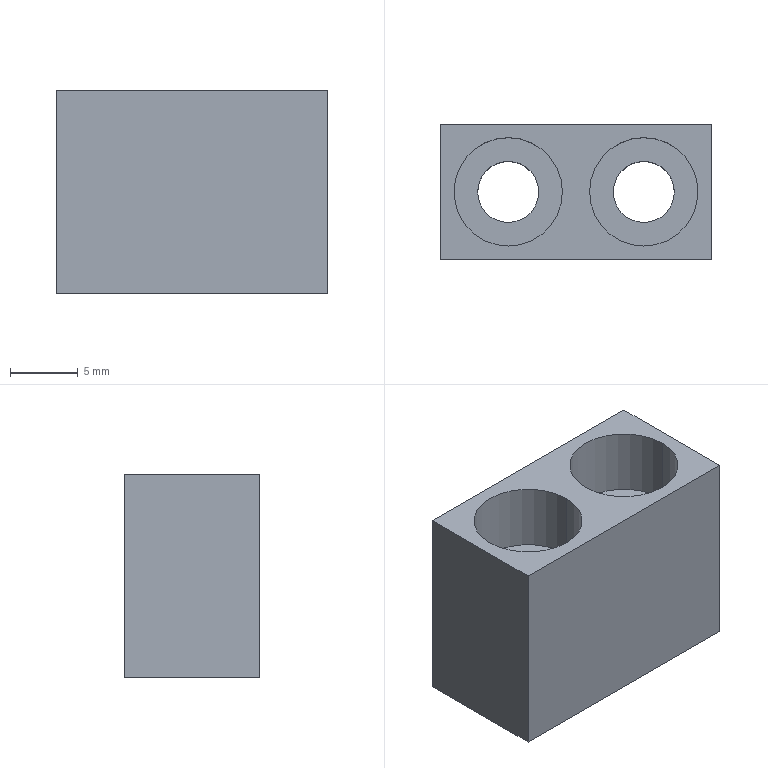Part | STEP file | 227H056259 Stop Block_Default | 1 solid | 16 faces | box 20 x 10 x 15 mm | volume 2179 mm3 | cylinder 8 | plane 8 | commonest cylinder face diameters 4.5 x4 8 x4
STEP:
#1=CARTESIAN_POINT('',(0.,0.,0.));
#2=DIRECTION('',(0.,0.,1.));
#3=DIRECTION('',(1.,0.,0.));
#4=AXIS2_PLACEMENT_3D('',#1,#2,#3);
#5=CARTESIAN_POINT('',(9.,5.,2.5));
#6=VERTEX_POINT('',#5);
#7=CARTESIAN_POINT('',(9.,5.,7.5));
#8=VERTEX_POINT('',#7);
#9=CARTESIAN_POINT('',(9.,5.,7.5));
#10=DIRECTION('',(0.,0.,1.));
#11=VECTOR('',#10,1.);
#12=LINE('',#9,#11);
#13=CARTESIAN_POINT('',(5.,5.,7.5));
#14=DIRECTION('',(0.,0.,1.));
#15=DIRECTION('',(1.,0.,0.));
#16=AXIS2_PLACEMENT_3D('',#13,#14,#15);
#17=CYLINDRICAL_SURFACE('',#16,4.);
#18=CARTESIAN_POINT('',(6.283,0.));
#19=DIRECTION('',(0.,1.));
#20=VECTOR('',#19,1.);
#21=LINE('',#18,#20);
#22=(GEOMETRIC_REPRESENTATION_CONTEXT(2)PARAMETRIC_REPRESENTATION_CONTEXT()REPRESENTATION_CONTEXT('',''));
#23=DEFINITIONAL_REPRESENTATION('',(#21),#22);
#24=PCURVE('',#17,#23);
#25=CARTESIAN_POINT('',(5.,5.,7.5));
#26=DIRECTION('',(0.,0.,1.));
#27=DIRECTION('',(1.,0.,0.));
#28=AXIS2_PLACEMENT_3D('',#25,#26,#27);
#29=CYLINDRICAL_SURFACE('',#28,4.);
#30=CARTESIAN_POINT('',(0.,0.));
#31=DIRECTION('',(0.,1.));
#32=VECTOR('',#31,1.);
#33=LINE('',#30,#32);
#34=(GEOMETRIC_REPRESENTATION_CONTEXT(2)PARAMETRIC_REPRESENTATION_CONTEXT()REPRESENTATION_CONTEXT('',''));
#35=DEFINITIONAL_REPRESENTATION('',(#33),#34);
#36=PCURVE('',#29,#35);
#37=SURFACE_CURVE('',#12,(#24,#36),.PCURVE_S1.);
#38=EDGE_CURVE('',#6,#8,#37,.T.);
#39=ORIENTED_EDGE('',*,*,#38,.T.);
#40=CARTESIAN_POINT('',(1.,5.,7.5));
#41=VERTEX_POINT('',#40);
#42=CARTESIAN_POINT('',(5.,5.,7.5));
#43=DIRECTION('',(0.,0.,1.));
#44=DIRECTION('',(1.,0.,0.));
#45=AXIS2_PLACEMENT_3D('',#42,#43,#44);
#46=CIRCLE('',#45,4.);
#47=CARTESIAN_POINT('',(0.,0.));
#48=DIRECTION('',(1.,0.));
#49=VECTOR('',#48,1.);
#50=LINE('',#47,#49);
#51=(GEOMETRIC_REPRESENTATION_CONTEXT(2)PARAMETRIC_REPRESENTATION_CONTEXT()REPRESENTATION_CONTEXT('',''));
#52=DEFINITIONAL_REPRESENTATION('',(#50),#51);
#53=PCURVE('',#17,#52);
#54=CARTESIAN_POINT('',(10.,10.,7.5));
#55=DIRECTION('',(0.,0.,-1.));
#56=DIRECTION('',(-1.,0.,0.));
#57=AXIS2_PLACEMENT_3D('',#54,#55,#56);
#58=PLANE('',#57);
#59=CARTESIAN_POINT('',(1.,-5.));
#60=CARTESIAN_POINT('',(1.,1.928));
#61=CARTESIAN_POINT('',(7.,-1.536));
#62=CARTESIAN_POINT('',(13.,-5.));
#63=CARTESIAN_POINT('',(7.,-8.464));
#64=CARTESIAN_POINT('',(1.,-11.928));
#65=CARTESIAN_POINT('',(1.,-5.));
#66=(BOUNDED_CURVE()B_SPLINE_CURVE(2,(#59,#60,#61,#62,#63,#64,#65),.UNSPECIFIED.,.T.,.F.)B_SPLINE_CURVE_WITH_KNOTS((1,2,2,2,2,1),(-2.094,0.,2.094,4.189,6.283,8.378),.UNSPECIFIED.)CURVE()GEOMETRIC_REPRESENTATION_ITEM()RATIONAL_B_SPLINE_CURVE((1.,0.5,1.,0.5,1.,0.5,1.))REPRESENTATION_ITEM(''));
#67=(GEOMETRIC_REPRESENTATION_CONTEXT(2)PARAMETRIC_REPRESENTATION_CONTEXT()REPRESENTATION_CONTEXT('',''));
#68=DEFINITIONAL_REPRESENTATION('',(#66),#67);
#69=PCURVE('',#58,#68);
#70=SURFACE_CURVE('',#46,(#53,#69),.PCURVE_S1.);
#71=EDGE_CURVE('',#41,#8,#70,.T.);
#72=ORIENTED_EDGE('',*,*,#71,.F.);
#73=CARTESIAN_POINT('',(1.,5.,2.5));
#74=VERTEX_POINT('',#73);
#75=CARTESIAN_POINT('',(1.,5.,7.5));
#76=DIRECTION('',(0.,0.,1.));
#77=VECTOR('',#76,1.);
#78=LINE('',#75,#77);
#79=CARTESIAN_POINT('',(3.142,0.));
#80=DIRECTION('',(0.,1.));
#81=VECTOR('',#80,1.);
#82=LINE('',#79,#81);
#83=(GEOMETRIC_REPRESENTATION_CONTEXT(2)PARAMETRIC_REPRESENTATION_CONTEXT()REPRESENTATION_CONTEXT('',''));
#84=DEFINITIONAL_REPRESENTATION('',(#82),#83);
#85=PCURVE('',#17,#84);
#86=CARTESIAN_POINT('',(3.142,0.));
#87=DIRECTION('',(0.,1.));
#88=VECTOR('',#87,1.);
#89=LINE('',#86,#88);
#90=(GEOMETRIC_REPRESENTATION_CONTEXT(2)PARAMETRIC_REPRESENTATION_CONTEXT()REPRESENTATION_CONTEXT('',''));
#91=DEFINITIONAL_REPRESENTATION('',(#89),#90);
#92=PCURVE('',#29,#91);
#93=SURFACE_CURVE('',#78,(#85,#92),.PCURVE_S1.);
#94=EDGE_CURVE('',#74,#41,#93,.T.);
#95=ORIENTED_EDGE('',*,*,#94,.F.);
#96=CARTESIAN_POINT('',(5.,5.,2.5));
#97=DIRECTION('',(0.,0.,1.));
#98=DIRECTION('',(1.,0.,0.));
#99=AXIS2_PLACEMENT_3D('',#96,#97,#98);
#100=CIRCLE('',#99,4.);
#101=CARTESIAN_POINT('',(0.,-5.));
#102=DIRECTION('',(1.,0.));
#103=VECTOR('',#102,1.);
#104=LINE('',#101,#103);
#105=(GEOMETRIC_REPRESENTATION_CONTEXT(2)PARAMETRIC_REPRESENTATION_CONTEXT()REPRESENTATION_CONTEXT('',''));
#106=DEFINITIONAL_REPRESENTATION('',(#104),#105);
#107=PCURVE('',#17,#106);
#108=CARTESIAN_POINT('',(7.25,5.,2.5));
#109=DIRECTION('',(0.,0.,-1.));
#110=DIRECTION('',(-1.,0.,0.));
#111=AXIS2_PLACEMENT_3D('',#108,#109,#110);
#112=PLANE('',#111);
#113=CARTESIAN_POINT('',(-1.75,0.));
#114=CARTESIAN_POINT('',(-1.75,6.928));
#115=CARTESIAN_POINT('',(4.25,3.464));
#116=CARTESIAN_POINT('',(10.25,0.));
#117=CARTESIAN_POINT('',(4.25,-3.464));
#118=CARTESIAN_POINT('',(-1.75,-6.928));
#119=CARTESIAN_POINT('',(-1.75,0.));
#120=(BOUNDED_CURVE()B_SPLINE_CURVE(2,(#113,#114,#115,#116,#117,#118,#119),.UNSPECIFIED.,.T.,.F.)B_SPLINE_CURVE_WITH_KNOTS((1,2,2,2,2,1),(-2.094,0.,2.094,4.189,6.283,8.378),.UNSPECIFIED.)CURVE()GEOMETRIC_REPRESENTATION_ITEM()RATIONAL_B_SPLINE_CURVE((1.,0.5,1.,0.5,1.,0.5,1.))REPRESENTATION_ITEM(''));
#121=(GEOMETRIC_REPRESENTATION_CONTEXT(2)PARAMETRIC_REPRESENTATION_CONTEXT()REPRESENTATION_CONTEXT('',''));
#122=DEFINITIONAL_REPRESENTATION('',(#120),#121);
#123=PCURVE('',#112,#122);
#124=SURFACE_CURVE('',#100,(#107,#123),.PCURVE_S1.);
#125=EDGE_CURVE('',#74,#6,#124,.T.);
#126=ORIENTED_EDGE('',*,*,#125,.T.);
#127=EDGE_LOOP('',(#39,#72,#95,#126));
#128=FACE_BOUND('',#127,.F.);
#129=ADVANCED_FACE('',(#128),#17,.F.);
#130=CARTESIAN_POINT('',(7.25,5.,-7.5));
#131=VERTEX_POINT('',#130);
#132=CARTESIAN_POINT('',(7.25,5.,2.5));
#133=VERTEX_POINT('',#132);
#134=CARTESIAN_POINT('',(7.25,5.,7.5));
#135=DIRECTION('',(0.,0.,1.));
#136=VECTOR('',#135,1.);
#137=LINE('',#134,#136);
#138=CARTESIAN_POINT('',(5.,5.,7.5));
#139=DIRECTION('',(0.,0.,1.));
#140=DIRECTION('',(1.,0.,0.));
#141=AXIS2_PLACEMENT_3D('',#138,#139,#140);
#142=CYLINDRICAL_SURFACE('',#141,2.25);
#143=CARTESIAN_POINT('',(6.283,0.));
#144=DIRECTION('',(0.,1.));
#145=VECTOR('',#144,1.);
#146=LINE('',#143,#145);
#147=(GEOMETRIC_REPRESENTATION_CONTEXT(2)PARAMETRIC_REPRESENTATION_CONTEXT()REPRESENTATION_CONTEXT('',''));
#148=DEFINITIONAL_REPRESENTATION('',(#146),#147);
#149=PCURVE('',#142,#148);
#150=CARTESIAN_POINT('',(5.,5.,7.5));
#151=DIRECTION('',(0.,0.,1.));
#152=DIRECTION('',(1.,0.,0.));
#153=AXIS2_PLACEMENT_3D('',#150,#151,#152);
#154=CYLINDRICAL_SURFACE('',#153,2.25);
#155=CARTESIAN_POINT('',(0.,0.));
#156=DIRECTION('',(0.,1.));
#157=VECTOR('',#156,1.);
#158=LINE('',#155,#157);
#159=(GEOMETRIC_REPRESENTATION_CONTEXT(2)PARAMETRIC_REPRESENTATION_CONTEXT()REPRESENTATION_CONTEXT('',''));
#160=DEFINITIONAL_REPRESENTATION('',(#158),#159);
#161=PCURVE('',#154,#160);
#162=SURFACE_CURVE('',#137,(#149,#161),.PCURVE_S1.);
#163=EDGE_CURVE('',#131,#133,#162,.T.);
#164=ORIENTED_EDGE('',*,*,#163,.T.);
#165=CARTESIAN_POINT('',(2.75,5.,2.5));
#166=VERTEX_POINT('',#165);
#167=CARTESIAN_POINT('',(5.,5.,2.5));
#168=DIRECTION('',(0.,0.,1.));
#169=DIRECTION('',(1.,0.,0.));
#170=AXIS2_PLACEMENT_3D('',#167,#168,#169);
#171=CIRCLE('',#170,2.25);
#172=CARTESIAN_POINT('',(0.,-5.));
#173=DIRECTION('',(1.,0.));
#174=VECTOR('',#173,1.);
#175=LINE('',#172,#174);
#176=(GEOMETRIC_REPRESENTATION_CONTEXT(2)PARAMETRIC_REPRESENTATION_CONTEXT()REPRESENTATION_CONTEXT('',''));
#177=DEFINITIONAL_REPRESENTATION('',(#175),#176);
#178=PCURVE('',#142,#177);
#179=CARTESIAN_POINT('',(0.,0.));
#180=CARTESIAN_POINT('',(0.,3.897));
#181=CARTESIAN_POINT('',(3.375,1.949));
#182=CARTESIAN_POINT('',(6.75,0.));
#183=CARTESIAN_POINT('',(3.375,-1.949));
#184=CARTESIAN_POINT('',(0.,-3.897));
#185=CARTESIAN_POINT('',(0.,0.));
#186=(BOUNDED_CURVE()B_SPLINE_CURVE(2,(#179,#180,#181,#182,#183,#184,#185),.UNSPECIFIED.,.T.,.F.)B_SPLINE_CURVE_WITH_KNOTS((1,2,2,2,2,1),(-2.094,0.,2.094,4.189,6.283,8.378),.UNSPECIFIED.)CURVE()GEOMETRIC_REPRESENTATION_ITEM()RATIONAL_B_SPLINE_CURVE((1.,0.5,1.,0.5,1.,0.5,1.))REPRESENTATION_ITEM(''));
#187=(GEOMETRIC_REPRESENTATION_CONTEXT(2)PARAMETRIC_REPRESENTATION_CONTEXT()REPRESENTATION_CONTEXT('',''));
#188=DEFINITIONAL_REPRESENTATION('',(#186),#187);
#189=PCURVE('',#112,#188);
#190=SURFACE_CURVE('',#171,(#178,#189),.PCURVE_S1.);
#191=EDGE_CURVE('',#166,#133,#190,.T.);
#192=ORIENTED_EDGE('',*,*,#191,.F.);
#193=CARTESIAN_POINT('',(2.75,5.,-7.5));
#194=VERTEX_POINT('',#193);
#195=CARTESIAN_POINT('',(2.75,5.,7.5));
#196=DIRECTION('',(0.,0.,1.));
#197=VECTOR('',#196,1.);
#198=LINE('',#195,#197);
#199=CARTESIAN_POINT('',(3.142,0.));
#200=DIRECTION('',(0.,1.));
#201=VECTOR('',#200,1.);
#202=LINE('',#199,#201);
#203=(GEOMETRIC_REPRESENTATION_CONTEXT(2)PARAMETRIC_REPRESENTATION_CONTEXT()REPRESENTATION_CONTEXT('',''));
#204=DEFINITIONAL_REPRESENTATION('',(#202),#203);
#205=PCURVE('',#142,#204);
#206=CARTESIAN_POINT('',(3.142,0.));
#207=DIRECTION('',(0.,1.));
#208=VECTOR('',#207,1.);
#209=LINE('',#206,#208);
#210=(GEOMETRIC_REPRESENTATION_CONTEXT(2)PARAMETRIC_REPRESENTATION_CONTEXT()REPRESENTATION_CONTEXT('',''));
#211=DEFINITIONAL_REPRESENTATION('',(#209),#210);
#212=PCURVE('',#154,#211);
#213=SURFACE_CURVE('',#198,(#205,#212),.PCURVE_S1.);
#214=EDGE_CURVE('',#194,#166,#213,.T.);
#215=ORIENTED_EDGE('',*,*,#214,.F.);
#216=CARTESIAN_POINT('',(5.,5.,-7.5));
#217=DIRECTION('',(0.,0.,1.));
#218=DIRECTION('',(1.,0.,0.));
#219=AXIS2_PLACEMENT_3D('',#216,#217,#218);
#220=CIRCLE('',#219,2.25);
#221=CARTESIAN_POINT('',(0.,-15.));
#222=DIRECTION('',(1.,0.));
#223=VECTOR('',#222,1.);
#224=LINE('',#221,#223);
#225=(GEOMETRIC_REPRESENTATION_CONTEXT(2)PARAMETRIC_REPRESENTATION_CONTEXT()REPRESENTATION_CONTEXT('',''));
#226=DEFINITIONAL_REPRESENTATION('',(#224),#225);
#227=PCURVE('',#142,#226);
#228=CARTESIAN_POINT('',(10.,10.,-7.5));
#229=DIRECTION('',(0.,0.,1.));
#230=DIRECTION('',(1.,0.,0.));
#231=AXIS2_PLACEMENT_3D('',#228,#229,#230);
#232=PLANE('',#231);
#233=CARTESIAN_POINT('',(-5.,-5.));
#234=DIRECTION('',(1.,0.));
#235=AXIS2_PLACEMENT_2D('',#233,#234);
#236=CIRCLE('',#235,2.25);
#237=(GEOMETRIC_REPRESENTATION_CONTEXT(2)PARAMETRIC_REPRESENTATION_CONTEXT()REPRESENTATION_CONTEXT('',''));
#238=DEFINITIONAL_REPRESENTATION('',(#236),#237);
#239=PCURVE('',#232,#238);
#240=SURFACE_CURVE('',#220,(#227,#239),.PCURVE_S1.);
#241=EDGE_CURVE('',#194,#131,#240,.T.);
#242=ORIENTED_EDGE('',*,*,#241,.T.);
#243=EDGE_LOOP('',(#164,#192,#215,#242));
#244=FACE_BOUND('',#243,.F.);
#245=ADVANCED_FACE('',(#244),#142,.F.);
#246=CARTESIAN_POINT('',(-1.,5.,2.5));
#247=VERTEX_POINT('',#246);
#248=CARTESIAN_POINT('',(-1.,5.,7.5));
#249=VERTEX_POINT('',#248);
#250=CARTESIAN_POINT('',(-1.,5.,7.5));
#251=DIRECTION('',(0.,0.,1.));
#252=VECTOR('',#251,1.);
#253=LINE('',#250,#252);
#254=CARTESIAN_POINT('',(-5.,5.,7.5));
#255=DIRECTION('',(0.,0.,1.));
#256=DIRECTION('',(1.,0.,0.));
#257=AXIS2_PLACEMENT_3D('',#254,#255,#256);
#258=CYLINDRICAL_SURFACE('',#257,4.);
#259=CARTESIAN_POINT('',(6.283,0.));
#260=DIRECTION('',(0.,1.));
#261=VECTOR('',#260,1.);
#262=LINE('',#259,#261);
#263=(GEOMETRIC_REPRESENTATION_CONTEXT(2)PARAMETRIC_REPRESENTATION_CONTEXT()REPRESENTATION_CONTEXT('',''));
#264=DEFINITIONAL_REPRESENTATION('',(#262),#263);
#265=PCURVE('',#258,#264);
#266=CARTESIAN_POINT('',(-5.,5.,7.5));
#267=DIRECTION('',(0.,0.,1.));
#268=DIRECTION('',(1.,0.,0.));
#269=AXIS2_PLACEMENT_3D('',#266,#267,#268);
#270=CYLINDRICAL_SURFACE('',#269,4.);
#271=CARTESIAN_POINT('',(0.,0.));
#272=DIRECTION('',(0.,1.));
#273=VECTOR('',#272,1.);
#274=LINE('',#271,#273);
#275=(GEOMETRIC_REPRESENTATION_CONTEXT(2)PARAMETRIC_REPRESENTATION_CONTEXT()REPRESENTATION_CONTEXT('',''));
#276=DEFINITIONAL_REPRESENTATION('',(#274),#275);
#277=PCURVE('',#270,#276);
#278=SURFACE_CURVE('',#253,(#265,#277),.PCURVE_S1.);
#279=EDGE_CURVE('',#247,#249,#278,.T.);
#280=ORIENTED_EDGE('',*,*,#279,.T.);
#281=CARTESIAN_POINT('',(-9.,5.,7.5));
#282=VERTEX_POINT('',#281);
#283=CARTESIAN_POINT('',(-5.,5.,7.5));
#284=DIRECTION('',(0.,0.,1.));
#285=DIRECTION('',(1.,0.,0.));
#286=AXIS2_PLACEMENT_3D('',#283,#284,#285);
#287=CIRCLE('',#286,4.);
#288=CARTESIAN_POINT('',(0.,0.));
#289=DIRECTION('',(1.,0.));
#290=VECTOR('',#289,1.);
#291=LINE('',#288,#290);
#292=(GEOMETRIC_REPRESENTATION_CONTEXT(2)PARAMETRIC_REPRESENTATION_CONTEXT()REPRESENTATION_CONTEXT('',''));
#293=DEFINITIONAL_REPRESENTATION('',(#291),#292);
#294=PCURVE('',#258,#293);
#295=CARTESIAN_POINT('',(11.,-5.));
#296=CARTESIAN_POINT('',(11.,1.928));
#297=CARTESIAN_POINT('',(17.,-1.536));
#298=CARTESIAN_POINT('',(23.,-5.));
#299=CARTESIAN_POINT('',(17.,-8.464));
#300=CARTESIAN_POINT('',(11.,-11.928));
#301=CARTESIAN_POINT('',(11.,-5.));
#302=(BOUNDED_CURVE()B_SPLINE_CURVE(2,(#295,#296,#297,#298,#299,#300,#301),.UNSPECIFIED.,.T.,.F.)B_SPLINE_CURVE_WITH_KNOTS((1,2,2,2,2,1),(-2.094,0.,2.094,4.189,6.283,8.378),.UNSPECIFIED.)CURVE()GEOMETRIC_REPRESENTATION_ITEM()RATIONAL_B_SPLINE_CURVE((1.,0.5,1.,0.5,1.,0.5,1.))REPRESENTATION_ITEM(''));
#303=(GEOMETRIC_REPRESENTATION_CONTEXT(2)PARAMETRIC_REPRESENTATION_CONTEXT()REPRESENTATION_CONTEXT('',''));
#304=DEFINITIONAL_REPRESENTATION('',(#302),#303);
#305=PCURVE('',#58,#304);
#306=SURFACE_CURVE('',#287,(#294,#305),.PCURVE_S1.);
#307=EDGE_CURVE('',#282,#249,#306,.T.);
#308=ORIENTED_EDGE('',*,*,#307,.F.);
#309=CARTESIAN_POINT('',(-9.,5.,2.5));
#310=VERTEX_POINT('',#309);
#311=CARTESIAN_POINT('',(-9.,5.,7.5));
#312=DIRECTION('',(0.,0.,1.));
#313=VECTOR('',#312,1.);
#314=LINE('',#311,#313);
#315=CARTESIAN_POINT('',(3.142,0.));
#316=DIRECTION('',(0.,1.));
#317=VECTOR('',#316,1.);
#318=LINE('',#315,#317);
#319=(GEOMETRIC_REPRESENTATION_CONTEXT(2)PARAMETRIC_REPRESENTATION_CONTEXT()REPRESENTATION_CONTEXT('',''));
#320=DEFINITIONAL_REPRESENTATION('',(#318),#319);
#321=PCURVE('',#258,#320);
#322=CARTESIAN_POINT('',(3.142,0.));
#323=DIRECTION('',(0.,1.));
#324=VECTOR('',#323,1.);
#325=LINE('',#322,#324);
#326=(GEOMETRIC_REPRESENTATION_CONTEXT(2)PARAMETRIC_REPRESENTATION_CONTEXT()REPRESENTATION_CONTEXT('',''));
#327=DEFINITIONAL_REPRESENTATION('',(#325),#326);
#328=PCURVE('',#270,#327);
#329=SURFACE_CURVE('',#314,(#321,#328),.PCURVE_S1.);
#330=EDGE_CURVE('',#310,#282,#329,.T.);
#331=ORIENTED_EDGE('',*,*,#330,.F.);
#332=CARTESIAN_POINT('',(-5.,5.,2.5));
#333=DIRECTION('',(0.,0.,1.));
#334=DIRECTION('',(1.,0.,0.));
#335=AXIS2_PLACEMENT_3D('',#332,#333,#334);
#336=CIRCLE('',#335,4.);
#337=CARTESIAN_POINT('',(0.,-5.));
#338=DIRECTION('',(1.,0.));
#339=VECTOR('',#338,1.);
#340=LINE('',#337,#339);
#341=(GEOMETRIC_REPRESENTATION_CONTEXT(2)PARAMETRIC_REPRESENTATION_CONTEXT()REPRESENTATION_CONTEXT('',''));
#342=DEFINITIONAL_REPRESENTATION('',(#340),#341);
#343=PCURVE('',#258,#342);
#344=CARTESIAN_POINT('',(-2.75,5.,2.5));
#345=DIRECTION('',(0.,0.,-1.));
#346=DIRECTION('',(-1.,0.,0.));
#347=AXIS2_PLACEMENT_3D('',#344,#345,#346);
#348=PLANE('',#347);
#349=CARTESIAN_POINT('',(-1.75,0.));
#350=CARTESIAN_POINT('',(-1.75,6.928));
#351=CARTESIAN_POINT('',(4.25,3.464));
#352=CARTESIAN_POINT('',(10.25,0.));
#353=CARTESIAN_POINT('',(4.25,-3.464));
#354=CARTESIAN_POINT('',(-1.75,-6.928));
#355=CARTESIAN_POINT('',(-1.75,0.));
#356=(BOUNDED_CURVE()B_SPLINE_CURVE(2,(#349,#350,#351,#352,#353,#354,#355),.UNSPECIFIED.,.T.,.F.)B_SPLINE_CURVE_WITH_KNOTS((1,2,2,2,2,1),(-2.094,0.,2.094,4.189,6.283,8.378),.UNSPECIFIED.)CURVE()GEOMETRIC_REPRESENTATION_ITEM()RATIONAL_B_SPLINE_CURVE((1.,0.5,1.,0.5,1.,0.5,1.))REPRESENTATION_ITEM(''));
#357=(GEOMETRIC_REPRESENTATION_CONTEXT(2)PARAMETRIC_REPRESENTATION_CONTEXT()REPRESENTATION_CONTEXT('',''));
#358=DEFINITIONAL_REPRESENTATION('',(#356),#357);
#359=PCURVE('',#348,#358);
#360=SURFACE_CURVE('',#336,(#343,#359),.PCURVE_S1.);
#361=EDGE_CURVE('',#310,#247,#360,.T.);
#362=ORIENTED_EDGE('',*,*,#361,.T.);
#363=EDGE_LOOP('',(#280,#308,#331,#362));
#364=FACE_BOUND('',#363,.F.);
#365=ADVANCED_FACE('',(#364),#258,.F.);
#366=CARTESIAN_POINT('',(-2.75,5.,-7.5));
#367=VERTEX_POINT('',#366);
#368=CARTESIAN_POINT('',(-2.75,5.,2.5));
#369=VERTEX_POINT('',#368);
#370=CARTESIAN_POINT('',(-2.75,5.,7.5));
#371=DIRECTION('',(0.,0.,1.));
#372=VECTOR('',#371,1.);
#373=LINE('',#370,#372);
#374=CARTESIAN_POINT('',(-5.,5.,7.5));
#375=DIRECTION('',(0.,0.,1.));
#376=DIRECTION('',(1.,0.,0.));
#377=AXIS2_PLACEMENT_3D('',#374,#375,#376);
#378=CYLINDRICAL_SURFACE('',#377,2.25);
#379=CARTESIAN_POINT('',(6.283,0.));
#380=DIRECTION('',(0.,1.));
#381=VECTOR('',#380,1.);
#382=LINE('',#379,#381);
#383=(GEOMETRIC_REPRESENTATION_CONTEXT(2)PARAMETRIC_REPRESENTATION_CONTEXT()REPRESENTATION_CONTEXT('',''));
#384=DEFINITIONAL_REPRESENTATION('',(#382),#383);
#385=PCURVE('',#378,#384);
#386=CARTESIAN_POINT('',(-5.,5.,7.5));
#387=DIRECTION('',(0.,0.,1.));
#388=DIRECTION('',(1.,0.,0.));
#389=AXIS2_PLACEMENT_3D('',#386,#387,#388);
#390=CYLINDRICAL_SURFACE('',#389,2.25);
#391=CARTESIAN_POINT('',(0.,0.));
#392=DIRECTION('',(0.,1.));
#393=VECTOR('',#392,1.);
#394=LINE('',#391,#393);
#395=(GEOMETRIC_REPRESENTATION_CONTEXT(2)PARAMETRIC_REPRESENTATION_CONTEXT()REPRESENTATION_CONTEXT('',''));
#396=DEFINITIONAL_REPRESENTATION('',(#394),#395);
#397=PCURVE('',#390,#396);
#398=SURFACE_CURVE('',#373,(#385,#397),.PCURVE_S1.);
#399=EDGE_CURVE('',#367,#369,#398,.T.);
#400=ORIENTED_EDGE('',*,*,#399,.T.);
#401=CARTESIAN_POINT('',(-7.25,5.,2.5));
#402=VERTEX_POINT('',#401);
#403=CARTESIAN_POINT('',(-5.,5.,2.5));
#404=DIRECTION('',(0.,0.,1.));
#405=DIRECTION('',(1.,0.,0.));
#406=AXIS2_PLACEMENT_3D('',#403,#404,#405);
#407=CIRCLE('',#406,2.25);
#408=CARTESIAN_POINT('',(0.,-5.));
#409=DIRECTION('',(1.,0.));
#410=VECTOR('',#409,1.);
#411=LINE('',#408,#410);
#412=(GEOMETRIC_REPRESENTATION_CONTEXT(2)PARAMETRIC_REPRESENTATION_CONTEXT()REPRESENTATION_CONTEXT('',''));
#413=DEFINITIONAL_REPRESENTATION('',(#411),#412);
#414=PCURVE('',#378,#413);
#415=CARTESIAN_POINT('',(0.,0.));
#416=CARTESIAN_POINT('',(0.,3.897));
#417=CARTESIAN_POINT('',(3.375,1.949));
#418=CARTESIAN_POINT('',(6.75,0.));
#419=CARTESIAN_POINT('',(3.375,-1.949));
#420=CARTESIAN_POINT('',(0.,-3.897));
#421=CARTESIAN_POINT('',(0.,0.));
#422=(BOUNDED_CURVE()B_SPLINE_CURVE(2,(#415,#416,#417,#418,#419,#420,#421),.UNSPECIFIED.,.T.,.F.)B_SPLINE_CURVE_WITH_KNOTS((1,2,2,2,2,1),(-2.094,0.,2.094,4.189,6.283,8.378),.UNSPECIFIED.)CURVE()GEOMETRIC_REPRESENTATION_ITEM()RATIONAL_B_SPLINE_CURVE((1.,0.5,1.,0.5,1.,0.5,1.))REPRESENTATION_ITEM(''));
#423=(GEOMETRIC_REPRESENTATION_CONTEXT(2)PARAMETRIC_REPRESENTATION_CONTEXT()REPRESENTATION_CONTEXT('',''));
#424=DEFINITIONAL_REPRESENTATION('',(#422),#423);
#425=PCURVE('',#348,#424);
#426=SURFACE_CURVE('',#407,(#414,#425),.PCURVE_S1.);
#427=EDGE_CURVE('',#402,#369,#426,.T.);
#428=ORIENTED_EDGE('',*,*,#427,.F.);
#429=CARTESIAN_POINT('',(-7.25,5.,-7.5));
#430=VERTEX_POINT('',#429);
#431=CARTESIAN_POINT('',(-7.25,5.,7.5));
#432=DIRECTION('',(0.,0.,1.));
#433=VECTOR('',#432,1.);
#434=LINE('',#431,#433);
#435=CARTESIAN_POINT('',(3.142,0.));
#436=DIRECTION('',(0.,1.));
#437=VECTOR('',#436,1.);
#438=LINE('',#435,#437);
#439=(GEOMETRIC_REPRESENTATION_CONTEXT(2)PARAMETRIC_REPRESENTATION_CONTEXT()REPRESENTATION_CONTEXT('',''));
#440=DEFINITIONAL_REPRESENTATION('',(#438),#439);
#441=PCURVE('',#378,#440);
#442=CARTESIAN_POINT('',(3.142,0.));
#443=DIRECTION('',(0.,1.));
#444=VECTOR('',#443,1.);
#445=LINE('',#442,#444);
#446=(GEOMETRIC_REPRESENTATION_CONTEXT(2)PARAMETRIC_REPRESENTATION_CONTEXT()REPRESENTATION_CONTEXT('',''));
#447=DEFINITIONAL_REPRESENTATION('',(#445),#446);
#448=PCURVE('',#390,#447);
#449=SURFACE_CURVE('',#434,(#441,#448),.PCURVE_S1.);
#450=EDGE_CURVE('',#430,#402,#449,.T.);
#451=ORIENTED_EDGE('',*,*,#450,.F.);
#452=CARTESIAN_POINT('',(-5.,5.,-7.5));
#453=DIRECTION('',(0.,0.,1.));
#454=DIRECTION('',(1.,0.,0.));
#455=AXIS2_PLACEMENT_3D('',#452,#453,#454);
#456=CIRCLE('',#455,2.25);
#457=CARTESIAN_POINT('',(0.,-15.));
#458=DIRECTION('',(1.,0.));
#459=VECTOR('',#458,1.);
#460=LINE('',#457,#459);
#461=(GEOMETRIC_REPRESENTATION_CONTEXT(2)PARAMETRIC_REPRESENTATION_CONTEXT()REPRESENTATION_CONTEXT('',''));
#462=DEFINITIONAL_REPRESENTATION('',(#460),#461);
#463=PCURVE('',#378,#462);
#464=CARTESIAN_POINT('',(-15.,-5.));
#465=DIRECTION('',(1.,0.));
#466=AXIS2_PLACEMENT_2D('',#464,#465);
#467=CIRCLE('',#466,2.25);
#468=(GEOMETRIC_REPRESENTATION_CONTEXT(2)PARAMETRIC_REPRESENTATION_CONTEXT()REPRESENTATION_CONTEXT('',''));
#469=DEFINITIONAL_REPRESENTATION('',(#467),#468);
#470=PCURVE('',#232,#469);
#471=SURFACE_CURVE('',#456,(#463,#470),.PCURVE_S1.);
#472=EDGE_CURVE('',#430,#367,#471,.T.);
#473=ORIENTED_EDGE('',*,*,#472,.T.);
#474=EDGE_LOOP('',(#400,#428,#451,#473));
#475=FACE_BOUND('',#474,.F.);
#476=ADVANCED_FACE('',(#475),#378,.F.);
#477=CARTESIAN_POINT('',(-10.,0.,-7.5));
#478=VERTEX_POINT('',#477);
#479=CARTESIAN_POINT('',(-10.,0.,7.5));
#480=VERTEX_POINT('',#479);
#481=CARTESIAN_POINT('',(-10.,0.,7.5));
#482=DIRECTION('',(0.,0.,1.));
#483=VECTOR('',#482,1.);
#484=LINE('',#481,#483);
#485=CARTESIAN_POINT('',(-10.,10.,7.5));
#486=DIRECTION('',(1.,0.,0.));
#487=DIRECTION('',(0.,0.,-1.));
#488=AXIS2_PLACEMENT_3D('',#485,#486,#487);
#489=PLANE('',#488);
#490=CARTESIAN_POINT('',(0.,-10.));
#491=DIRECTION('',(-1.,0.));
#492=VECTOR('',#491,1.);
#493=LINE('',#490,#492);
#494=(GEOMETRIC_REPRESENTATION_CONTEXT(2)PARAMETRIC_REPRESENTATION_CONTEXT()REPRESENTATION_CONTEXT('',''));
#495=DEFINITIONAL_REPRESENTATION('',(#493),#494);
#496=PCURVE('',#489,#495);
#497=CARTESIAN_POINT('',(0.,0.,0.));
#498=DIRECTION('',(0.,1.,0.));
#499=DIRECTION('',(0.,0.,1.));
#500=AXIS2_PLACEMENT_3D('',#497,#498,#499);
#501=PLANE('',#500);
#502=CARTESIAN_POINT('',(7.5,-10.));
#503=DIRECTION('',(1.,0.));
#504=VECTOR('',#503,1.);
#505=LINE('',#502,#504);
#506=(GEOMETRIC_REPRESENTATION_CONTEXT(2)PARAMETRIC_REPRESENTATION_CONTEXT()REPRESENTATION_CONTEXT('',''));
#507=DEFINITIONAL_REPRESENTATION('',(#505),#506);
#508=PCURVE('',#501,#507);
#509=SURFACE_CURVE('',#484,(#496,#508),.PCURVE_S1.);
#510=EDGE_CURVE('',#478,#480,#509,.T.);
#511=ORIENTED_EDGE('',*,*,#510,.T.);
#512=CARTESIAN_POINT('',(-10.,10.,7.5));
#513=VERTEX_POINT('',#512);
#514=CARTESIAN_POINT('',(-10.,10.,7.5));
#515=DIRECTION('',(0.,-1.,0.));
#516=VECTOR('',#515,1.);
#517=LINE('',#514,#516);
#518=CARTESIAN_POINT('',(0.,0.));
#519=DIRECTION('',(0.,-1.));
#520=VECTOR('',#519,1.);
#521=LINE('',#518,#520);
#522=(GEOMETRIC_REPRESENTATION_CONTEXT(2)PARAMETRIC_REPRESENTATION_CONTEXT()REPRESENTATION_CONTEXT('',''));
#523=DEFINITIONAL_REPRESENTATION('',(#521),#522);
#524=PCURVE('',#489,#523);
#525=CARTESIAN_POINT('',(20.,0.));
#526=DIRECTION('',(0.,-1.));
#527=VECTOR('',#526,1.);
#528=LINE('',#525,#527);
#529=(GEOMETRIC_REPRESENTATION_CONTEXT(2)PARAMETRIC_REPRESENTATION_CONTEXT()REPRESENTATION_CONTEXT('',''));
#530=DEFINITIONAL_REPRESENTATION('',(#528),#529);
#531=PCURVE('',#58,#530);
#532=SURFACE_CURVE('',#517,(#524,#531),.PCURVE_S1.);
#533=EDGE_CURVE('',#513,#480,#532,.T.);
#534=ORIENTED_EDGE('',*,*,#533,.F.);
#535=CARTESIAN_POINT('',(-10.,10.,-7.5));
#536=VERTEX_POINT('',#535);
#537=CARTESIAN_POINT('',(-10.,10.,7.5));
#538=DIRECTION('',(0.,0.,1.));
#539=VECTOR('',#538,1.);
#540=LINE('',#537,#539);
#541=CARTESIAN_POINT('',(0.,0.));
#542=DIRECTION('',(-1.,0.));
#543=VECTOR('',#542,1.);
#544=LINE('',#541,#543);
#545=(GEOMETRIC_REPRESENTATION_CONTEXT(2)PARAMETRIC_REPRESENTATION_CONTEXT()REPRESENTATION_CONTEXT('',''));
#546=DEFINITIONAL_REPRESENTATION('',(#544),#545);
#547=PCURVE('',#489,#546);
#548=CARTESIAN_POINT('',(0.,10.,0.));
#549=DIRECTION('',(0.,1.,0.));
#550=DIRECTION('',(0.,0.,1.));
#551=AXIS2_PLACEMENT_3D('',#548,#549,#550);
#552=PLANE('',#551);
#553=CARTESIAN_POINT('',(7.5,-10.));
#554=DIRECTION('',(1.,0.));
#555=VECTOR('',#554,1.);
#556=LINE('',#553,#555);
#557=(GEOMETRIC_REPRESENTATION_CONTEXT(2)PARAMETRIC_REPRESENTATION_CONTEXT()REPRESENTATION_CONTEXT('',''));
#558=DEFINITIONAL_REPRESENTATION('',(#556),#557);
#559=PCURVE('',#552,#558);
#560=SURFACE_CURVE('',#540,(#547,#559),.PCURVE_S1.);
#561=EDGE_CURVE('',#536,#513,#560,.T.);
#562=ORIENTED_EDGE('',*,*,#561,.F.);
#563=CARTESIAN_POINT('',(-10.,10.,-7.5));
#564=DIRECTION('',(0.,-1.,0.));
#565=VECTOR('',#564,1.);
#566=LINE('',#563,#565);
#567=CARTESIAN_POINT('',(15.,0.));
#568=DIRECTION('',(0.,-1.));
#569=VECTOR('',#568,1.);
#570=LINE('',#567,#569);
#571=(GEOMETRIC_REPRESENTATION_CONTEXT(2)PARAMETRIC_REPRESENTATION_CONTEXT()REPRESENTATION_CONTEXT('',''));
#572=DEFINITIONAL_REPRESENTATION('',(#570),#571);
#573=PCURVE('',#489,#572);
#574=CARTESIAN_POINT('',(-20.,0.));
#575=DIRECTION('',(0.,-1.));
#576=VECTOR('',#575,1.);
#577=LINE('',#574,#576);
#578=(GEOMETRIC_REPRESENTATION_CONTEXT(2)PARAMETRIC_REPRESENTATION_CONTEXT()REPRESENTATION_CONTEXT('',''));
#579=DEFINITIONAL_REPRESENTATION('',(#577),#578);
#580=PCURVE('',#232,#579);
#581=SURFACE_CURVE('',#566,(#573,#580),.PCURVE_S1.);
#582=EDGE_CURVE('',#536,#478,#581,.T.);
#583=ORIENTED_EDGE('',*,*,#582,.T.);
#584=EDGE_LOOP('',(#511,#534,#562,#583));
#585=FACE_BOUND('',#584,.T.);
#586=ADVANCED_FACE('',(#585),#489,.F.);
#587=CARTESIAN_POINT('',(5.,5.,7.5));
#588=DIRECTION('',(0.,0.,1.));
#589=DIRECTION('',(1.,0.,0.));
#590=AXIS2_PLACEMENT_3D('',#587,#588,#589);
#591=CIRCLE('',#590,4.);
#592=CARTESIAN_POINT('',(1.,-5.));
#593=CARTESIAN_POINT('',(1.,1.928));
#594=CARTESIAN_POINT('',(7.,-1.536));
#595=CARTESIAN_POINT('',(13.,-5.));
#596=CARTESIAN_POINT('',(7.,-8.464));
#597=CARTESIAN_POINT('',(1.,-11.928));
#598=CARTESIAN_POINT('',(1.,-5.));
#599=(BOUNDED_CURVE()B_SPLINE_CURVE(2,(#592,#593,#594,#595,#596,#597,#598),.UNSPECIFIED.,.T.,.F.)B_SPLINE_CURVE_WITH_KNOTS((1,2,2,2,2,1),(-2.094,0.,2.094,4.189,6.283,8.378),.UNSPECIFIED.)CURVE()GEOMETRIC_REPRESENTATION_ITEM()RATIONAL_B_SPLINE_CURVE((1.,0.5,1.,0.5,1.,0.5,1.))REPRESENTATION_ITEM(''));
#600=(GEOMETRIC_REPRESENTATION_CONTEXT(2)PARAMETRIC_REPRESENTATION_CONTEXT()REPRESENTATION_CONTEXT('',''));
#601=DEFINITIONAL_REPRESENTATION('',(#599),#600);
#602=PCURVE('',#58,#601);
#603=CARTESIAN_POINT('',(0.,0.));
#604=DIRECTION('',(1.,0.));
#605=VECTOR('',#604,1.);
#606=LINE('',#603,#605);
#607=(GEOMETRIC_REPRESENTATION_CONTEXT(2)PARAMETRIC_REPRESENTATION_CONTEXT()REPRESENTATION_CONTEXT('',''));
#608=DEFINITIONAL_REPRESENTATION('',(#606),#607);
#609=PCURVE('',#29,#608);
#610=SURFACE_CURVE('',#591,(#602,#609),.PCURVE_S1.);
#611=EDGE_CURVE('',#8,#41,#610,.T.);
#612=ORIENTED_EDGE('',*,*,#611,.F.);
#613=ORIENTED_EDGE('',*,*,#71,.F.);
#614=EDGE_LOOP('',(#612,#613));
#615=FACE_BOUND('',#614,.T.);
#616=CARTESIAN_POINT('',(-5.,5.,7.5));
#617=DIRECTION('',(0.,0.,1.));
#618=DIRECTION('',(1.,0.,0.));
#619=AXIS2_PLACEMENT_3D('',#616,#617,#618);
#620=CIRCLE('',#619,4.);
#621=CARTESIAN_POINT('',(11.,-5.));
#622=CARTESIAN_POINT('',(11.,1.928));
#623=CARTESIAN_POINT('',(17.,-1.536));
#624=CARTESIAN_POINT('',(23.,-5.));
#625=CARTESIAN_POINT('',(17.,-8.464));
#626=CARTESIAN_POINT('',(11.,-11.928));
#627=CARTESIAN_POINT('',(11.,-5.));
#628=(BOUNDED_CURVE()B_SPLINE_CURVE(2,(#621,#622,#623,#624,#625,#626,#627),.UNSPECIFIED.,.T.,.F.)B_SPLINE_CURVE_WITH_KNOTS((1,2,2,2,2,1),(-2.094,0.,2.094,4.189,6.283,8.378),.UNSPECIFIED.)CURVE()GEOMETRIC_REPRESENTATION_ITEM()RATIONAL_B_SPLINE_CURVE((1.,0.5,1.,0.5,1.,0.5,1.))REPRESENTATION_ITEM(''));
#629=(GEOMETRIC_REPRESENTATION_CONTEXT(2)PARAMETRIC_REPRESENTATION_CONTEXT()REPRESENTATION_CONTEXT('',''));
#630=DEFINITIONAL_REPRESENTATION('',(#628),#629);
#631=PCURVE('',#58,#630);
#632=CARTESIAN_POINT('',(0.,0.));
#633=DIRECTION('',(1.,0.));
#634=VECTOR('',#633,1.);
#635=LINE('',#632,#634);
#636=(GEOMETRIC_REPRESENTATION_CONTEXT(2)PARAMETRIC_REPRESENTATION_CONTEXT()REPRESENTATION_CONTEXT('',''));
#637=DEFINITIONAL_REPRESENTATION('',(#635),#636);
#638=PCURVE('',#270,#637);
#639=SURFACE_CURVE('',#620,(#631,#638),.PCURVE_S1.);
#640=EDGE_CURVE('',#249,#282,#639,.T.);
#641=ORIENTED_EDGE('',*,*,#640,.F.);
#642=ORIENTED_EDGE('',*,*,#307,.F.);
#643=EDGE_LOOP('',(#641,#642));
#644=FACE_BOUND('',#643,.T.);
#645=CARTESIAN_POINT('',(10.,0.,7.5));
#646=VERTEX_POINT('',#645);
#647=CARTESIAN_POINT('',(10.,0.,7.5));
#648=DIRECTION('',(1.,0.,0.));
#649=VECTOR('',#648,1.);
#650=LINE('',#647,#649);
#651=CARTESIAN_POINT('',(0.,-10.));
#652=DIRECTION('',(-1.,0.));
#653=VECTOR('',#652,1.);
#654=LINE('',#651,#653);
#655=(GEOMETRIC_REPRESENTATION_CONTEXT(2)PARAMETRIC_REPRESENTATION_CONTEXT()REPRESENTATION_CONTEXT('',''));
#656=DEFINITIONAL_REPRESENTATION('',(#654),#655);
#657=PCURVE('',#58,#656);
#658=CARTESIAN_POINT('',(7.5,10.));
#659=DIRECTION('',(0.,1.));
#660=VECTOR('',#659,1.);
#661=LINE('',#658,#660);
#662=(GEOMETRIC_REPRESENTATION_CONTEXT(2)PARAMETRIC_REPRESENTATION_CONTEXT()REPRESENTATION_CONTEXT('',''));
#663=DEFINITIONAL_REPRESENTATION('',(#661),#662);
#664=PCURVE('',#501,#663);
#665=SURFACE_CURVE('',#650,(#657,#664),.PCURVE_S1.);
#666=EDGE_CURVE('',#480,#646,#665,.T.);
#667=ORIENTED_EDGE('',*,*,#666,.T.);
#668=CARTESIAN_POINT('',(10.,10.,7.5));
#669=VERTEX_POINT('',#668);
#670=CARTESIAN_POINT('',(10.,10.,7.5));
#671=DIRECTION('',(0.,-1.,0.));
#672=VECTOR('',#671,1.);
#673=LINE('',#670,#672);
#674=CARTESIAN_POINT('',(0.,0.));
#675=DIRECTION('',(0.,-1.));
#676=VECTOR('',#675,1.);
#677=LINE('',#674,#676);
#678=(GEOMETRIC_REPRESENTATION_CONTEXT(2)PARAMETRIC_REPRESENTATION_CONTEXT()REPRESENTATION_CONTEXT('',''));
#679=DEFINITIONAL_REPRESENTATION('',(#677),#678);
#680=PCURVE('',#58,#679);
#681=CARTESIAN_POINT('',(10.,10.,7.5));
#682=DIRECTION('',(-1.,0.,0.));
#683=DIRECTION('',(0.,0.,1.));
#684=AXIS2_PLACEMENT_3D('',#681,#682,#683);
#685=PLANE('',#684);
#686=CARTESIAN_POINT('',(0.,0.));
#687=DIRECTION('',(0.,-1.));
#688=VECTOR('',#687,1.);
#689=LINE('',#686,#688);
#690=(GEOMETRIC_REPRESENTATION_CONTEXT(2)PARAMETRIC_REPRESENTATION_CONTEXT()REPRESENTATION_CONTEXT('',''));
#691=DEFINITIONAL_REPRESENTATION('',(#689),#690);
#692=PCURVE('',#685,#691);
#693=SURFACE_CURVE('',#673,(#680,#692),.PCURVE_S1.);
#694=EDGE_CURVE('',#669,#646,#693,.T.);
#695=ORIENTED_EDGE('',*,*,#694,.F.);
#696=CARTESIAN_POINT('',(10.,10.,7.5));
#697=DIRECTION('',(1.,0.,0.));
#698=VECTOR('',#697,1.);
#699=LINE('',#696,#698);
#700=CARTESIAN_POINT('',(0.,0.));
#701=DIRECTION('',(-1.,0.));
#702=VECTOR('',#701,1.);
#703=LINE('',#700,#702);
#704=(GEOMETRIC_REPRESENTATION_CONTEXT(2)PARAMETRIC_REPRESENTATION_CONTEXT()REPRESENTATION_CONTEXT('',''));
#705=DEFINITIONAL_REPRESENTATION('',(#703),#704);
#706=PCURVE('',#58,#705);
#707=CARTESIAN_POINT('',(7.5,10.));
#708=DIRECTION('',(0.,1.));
#709=VECTOR('',#708,1.);
#710=LINE('',#707,#709);
#711=(GEOMETRIC_REPRESENTATION_CONTEXT(2)PARAMETRIC_REPRESENTATION_CONTEXT()REPRESENTATION_CONTEXT('',''));
#712=DEFINITIONAL_REPRESENTATION('',(#710),#711);
#713=PCURVE('',#552,#712);
#714=SURFACE_CURVE('',#699,(#706,#713),.PCURVE_S1.);
#715=EDGE_CURVE('',#513,#669,#714,.T.);
#716=ORIENTED_EDGE('',*,*,#715,.F.);
#717=ORIENTED_EDGE('',*,*,#533,.T.);
#718=EDGE_LOOP('',(#667,#695,#716,#717));
#719=FACE_BOUND('',#718,.T.);
#720=ADVANCED_FACE('',(#615,#644,#719),#58,.F.);
#721=CARTESIAN_POINT('',(10.,0.,-7.5));
#722=VERTEX_POINT('',#721);
#723=CARTESIAN_POINT('',(10.,0.,7.5));
#724=DIRECTION('',(0.,0.,-1.));
#725=VECTOR('',#724,1.);
#726=LINE('',#723,#725);
#727=CARTESIAN_POINT('',(0.,-10.));
#728=DIRECTION('',(-1.,0.));
#729=VECTOR('',#728,1.);
#730=LINE('',#727,#729);
#731=(GEOMETRIC_REPRESENTATION_CONTEXT(2)PARAMETRIC_REPRESENTATION_CONTEXT()REPRESENTATION_CONTEXT('',''));
#732=DEFINITIONAL_REPRESENTATION('',(#730),#731);
#733=PCURVE('',#685,#732);
#734=CARTESIAN_POINT('',(7.5,10.));
#735=DIRECTION('',(-1.,0.));
#736=VECTOR('',#735,1.);
#737=LINE('',#734,#736);
#738=(GEOMETRIC_REPRESENTATION_CONTEXT(2)PARAMETRIC_REPRESENTATION_CONTEXT()REPRESENTATION_CONTEXT('',''));
#739=DEFINITIONAL_REPRESENTATION('',(#737),#738);
#740=PCURVE('',#501,#739);
#741=SURFACE_CURVE('',#726,(#733,#740),.PCURVE_S1.);
#742=EDGE_CURVE('',#646,#722,#741,.T.);
#743=ORIENTED_EDGE('',*,*,#742,.T.);
#744=CARTESIAN_POINT('',(10.,10.,-7.5));
#745=VERTEX_POINT('',#744);
#746=CARTESIAN_POINT('',(10.,10.,-7.5));
#747=DIRECTION('',(0.,-1.,0.));
#748=VECTOR('',#747,1.);
#749=LINE('',#746,#748);
#750=CARTESIAN_POINT('',(-15.,0.));
#751=DIRECTION('',(0.,-1.));
#752=VECTOR('',#751,1.);
#753=LINE('',#750,#752);
#754=(GEOMETRIC_REPRESENTATION_CONTEXT(2)PARAMETRIC_REPRESENTATION_CONTEXT()REPRESENTATION_CONTEXT('',''));
#755=DEFINITIONAL_REPRESENTATION('',(#753),#754);
#756=PCURVE('',#685,#755);
#757=CARTESIAN_POINT('',(0.,0.));
#758=DIRECTION('',(0.,-1.));
#759=VECTOR('',#758,1.);
#760=LINE('',#757,#759);
#761=(GEOMETRIC_REPRESENTATION_CONTEXT(2)PARAMETRIC_REPRESENTATION_CONTEXT()REPRESENTATION_CONTEXT('',''));
#762=DEFINITIONAL_REPRESENTATION('',(#760),#761);
#763=PCURVE('',#232,#762);
#764=SURFACE_CURVE('',#749,(#756,#763),.PCURVE_S1.);
#765=EDGE_CURVE('',#745,#722,#764,.T.);
#766=ORIENTED_EDGE('',*,*,#765,.F.);
#767=CARTESIAN_POINT('',(10.,10.,7.5));
#768=DIRECTION('',(0.,0.,-1.));
#769=VECTOR('',#768,1.);
#770=LINE('',#767,#769);
#771=CARTESIAN_POINT('',(0.,0.));
#772=DIRECTION('',(-1.,0.));
#773=VECTOR('',#772,1.);
#774=LINE('',#771,#773);
#775=(GEOMETRIC_REPRESENTATION_CONTEXT(2)PARAMETRIC_REPRESENTATION_CONTEXT()REPRESENTATION_CONTEXT('',''));
#776=DEFINITIONAL_REPRESENTATION('',(#774),#775);
#777=PCURVE('',#685,#776);
#778=CARTESIAN_POINT('',(7.5,10.));
#779=DIRECTION('',(-1.,0.));
#780=VECTOR('',#779,1.);
#781=LINE('',#778,#780);
#782=(GEOMETRIC_REPRESENTATION_CONTEXT(2)PARAMETRIC_REPRESENTATION_CONTEXT()REPRESENTATION_CONTEXT('',''));
#783=DEFINITIONAL_REPRESENTATION('',(#781),#782);
#784=PCURVE('',#552,#783);
#785=SURFACE_CURVE('',#770,(#777,#784),.PCURVE_S1.);
#786=EDGE_CURVE('',#669,#745,#785,.T.);
#787=ORIENTED_EDGE('',*,*,#786,.F.);
#788=ORIENTED_EDGE('',*,*,#694,.T.);
#789=EDGE_LOOP('',(#743,#766,#787,#788));
#790=FACE_BOUND('',#789,.T.);
#791=ADVANCED_FACE('',(#790),#685,.F.);
#792=CARTESIAN_POINT('',(5.,5.,-7.5));
#793=DIRECTION('',(0.,0.,1.));
#794=DIRECTION('',(1.,0.,0.));
#795=AXIS2_PLACEMENT_3D('',#792,#793,#794);
#796=CIRCLE('',#795,2.25);
#797=CARTESIAN_POINT('',(-5.,-5.));
#798=DIRECTION('',(1.,0.));
#799=AXIS2_PLACEMENT_2D('',#797,#798);
#800=CIRCLE('',#799,2.25);
#801=(GEOMETRIC_REPRESENTATION_CONTEXT(2)PARAMETRIC_REPRESENTATION_CONTEXT()REPRESENTATION_CONTEXT('',''));
#802=DEFINITIONAL_REPRESENTATION('',(#800),#801);
#803=PCURVE('',#232,#802);
#804=CARTESIAN_POINT('',(0.,-15.));
#805=DIRECTION('',(1.,0.));
#806=VECTOR('',#805,1.);
#807=LINE('',#804,#806);
#808=(GEOMETRIC_REPRESENTATION_CONTEXT(2)PARAMETRIC_REPRESENTATION_CONTEXT()REPRESENTATION_CONTEXT('',''));
#809=DEFINITIONAL_REPRESENTATION('',(#807),#808);
#810=PCURVE('',#154,#809);
#811=SURFACE_CURVE('',#796,(#803,#810),.PCURVE_S1.);
#812=EDGE_CURVE('',#131,#194,#811,.T.);
#813=ORIENTED_EDGE('',*,*,#812,.T.);
#814=ORIENTED_EDGE('',*,*,#241,.T.);
#815=EDGE_LOOP('',(#813,#814));
#816=FACE_BOUND('',#815,.T.);
#817=CARTESIAN_POINT('',(-5.,5.,-7.5));
#818=DIRECTION('',(0.,0.,1.));
#819=DIRECTION('',(1.,0.,0.));
#820=AXIS2_PLACEMENT_3D('',#817,#818,#819);
#821=CIRCLE('',#820,2.25);
#822=CARTESIAN_POINT('',(-15.,-5.));
#823=DIRECTION('',(1.,0.));
#824=AXIS2_PLACEMENT_2D('',#822,#823);
#825=CIRCLE('',#824,2.25);
#826=(GEOMETRIC_REPRESENTATION_CONTEXT(2)PARAMETRIC_REPRESENTATION_CONTEXT()REPRESENTATION_CONTEXT('',''));
#827=DEFINITIONAL_REPRESENTATION('',(#825),#826);
#828=PCURVE('',#232,#827);
#829=CARTESIAN_POINT('',(0.,-15.));
#830=DIRECTION('',(1.,0.));
#831=VECTOR('',#830,1.);
#832=LINE('',#829,#831);
#833=(GEOMETRIC_REPRESENTATION_CONTEXT(2)PARAMETRIC_REPRESENTATION_CONTEXT()REPRESENTATION_CONTEXT('',''));
#834=DEFINITIONAL_REPRESENTATION('',(#832),#833);
#835=PCURVE('',#390,#834);
#836=SURFACE_CURVE('',#821,(#828,#835),.PCURVE_S1.);
#837=EDGE_CURVE('',#367,#430,#836,.T.);
#838=ORIENTED_EDGE('',*,*,#837,.T.);
#839=ORIENTED_EDGE('',*,*,#472,.T.);
#840=EDGE_LOOP('',(#838,#839));
#841=FACE_BOUND('',#840,.T.);
#842=CARTESIAN_POINT('',(10.,0.,-7.5));
#843=DIRECTION('',(-1.,0.,0.));
#844=VECTOR('',#843,1.);
#845=LINE('',#842,#844);
#846=CARTESIAN_POINT('',(0.,-10.));
#847=DIRECTION('',(-1.,0.));
#848=VECTOR('',#847,1.);
#849=LINE('',#846,#848);
#850=(GEOMETRIC_REPRESENTATION_CONTEXT(2)PARAMETRIC_REPRESENTATION_CONTEXT()REPRESENTATION_CONTEXT('',''));
#851=DEFINITIONAL_REPRESENTATION('',(#849),#850);
#852=PCURVE('',#232,#851);
#853=CARTESIAN_POINT('',(-7.5,10.));
#854=DIRECTION('',(0.,-1.));
#855=VECTOR('',#854,1.);
#856=LINE('',#853,#855);
#857=(GEOMETRIC_REPRESENTATION_CONTEXT(2)PARAMETRIC_REPRESENTATION_CONTEXT()REPRESENTATION_CONTEXT('',''));
#858=DEFINITIONAL_REPRESENTATION('',(#856),#857);
#859=PCURVE('',#501,#858);
#860=SURFACE_CURVE('',#845,(#852,#859),.PCURVE_S1.);
#861=EDGE_CURVE('',#722,#478,#860,.T.);
#862=ORIENTED_EDGE('',*,*,#861,.T.);
#863=ORIENTED_EDGE('',*,*,#582,.F.);
#864=CARTESIAN_POINT('',(10.,10.,-7.5));
#865=DIRECTION('',(-1.,0.,0.));
#866=VECTOR('',#865,1.);
#867=LINE('',#864,#866);
#868=CARTESIAN_POINT('',(0.,0.));
#869=DIRECTION('',(-1.,0.));
#870=VECTOR('',#869,1.);
#871=LINE('',#868,#870);
#872=(GEOMETRIC_REPRESENTATION_CONTEXT(2)PARAMETRIC_REPRESENTATION_CONTEXT()REPRESENTATION_CONTEXT('',''));
#873=DEFINITIONAL_REPRESENTATION('',(#871),#872);
#874=PCURVE('',#232,#873);
#875=CARTESIAN_POINT('',(-7.5,10.));
#876=DIRECTION('',(0.,-1.));
#877=VECTOR('',#876,1.);
#878=LINE('',#875,#877);
#879=(GEOMETRIC_REPRESENTATION_CONTEXT(2)PARAMETRIC_REPRESENTATION_CONTEXT()REPRESENTATION_CONTEXT('',''));
#880=DEFINITIONAL_REPRESENTATION('',(#878),#879);
#881=PCURVE('',#552,#880);
#882=SURFACE_CURVE('',#867,(#874,#881),.PCURVE_S1.);
#883=EDGE_CURVE('',#745,#536,#882,.T.);
#884=ORIENTED_EDGE('',*,*,#883,.F.);
#885=ORIENTED_EDGE('',*,*,#765,.T.);
#886=EDGE_LOOP('',(#862,#863,#884,#885));
#887=FACE_BOUND('',#886,.T.);
#888=ADVANCED_FACE('',(#816,#841,#887),#232,.F.);
#889=ORIENTED_EDGE('',*,*,#561,.T.);
#890=ORIENTED_EDGE('',*,*,#715,.T.);
#891=ORIENTED_EDGE('',*,*,#786,.T.);
#892=ORIENTED_EDGE('',*,*,#883,.T.);
#893=EDGE_LOOP('',(#889,#890,#891,#892));
#894=FACE_BOUND('',#893,.T.);
#895=ADVANCED_FACE('',(#894),#552,.T.);
#896=ORIENTED_EDGE('',*,*,#510,.F.);
#897=ORIENTED_EDGE('',*,*,#861,.F.);
#898=ORIENTED_EDGE('',*,*,#742,.F.);
#899=ORIENTED_EDGE('',*,*,#666,.F.);
#900=EDGE_LOOP('',(#896,#897,#898,#899));
#901=FACE_BOUND('',#900,.T.);
#902=ADVANCED_FACE('',(#901),#501,.F.);
#903=CARTESIAN_POINT('',(-5.,5.,2.5));
#904=DIRECTION('',(0.,0.,1.));
#905=DIRECTION('',(1.,0.,0.));
#906=AXIS2_PLACEMENT_3D('',#903,#904,#905);
#907=CIRCLE('',#906,2.25);
#908=CARTESIAN_POINT('',(0.,-5.));
#909=DIRECTION('',(1.,0.));
#910=VECTOR('',#909,1.);
#911=LINE('',#908,#910);
#912=(GEOMETRIC_REPRESENTATION_CONTEXT(2)PARAMETRIC_REPRESENTATION_CONTEXT()REPRESENTATION_CONTEXT('',''));
#913=DEFINITIONAL_REPRESENTATION('',(#911),#912);
#914=PCURVE('',#390,#913);
#915=CARTESIAN_POINT('',(0.,0.));
#916=CARTESIAN_POINT('',(0.,3.897));
#917=CARTESIAN_POINT('',(3.375,1.949));
#918=CARTESIAN_POINT('',(6.75,0.));
#919=CARTESIAN_POINT('',(3.375,-1.949));
#920=CARTESIAN_POINT('',(0.,-3.897));
#921=CARTESIAN_POINT('',(0.,0.));
#922=(BOUNDED_CURVE()B_SPLINE_CURVE(2,(#915,#916,#917,#918,#919,#920,#921),.UNSPECIFIED.,.T.,.F.)B_SPLINE_CURVE_WITH_KNOTS((1,2,2,2,2,1),(-2.094,0.,2.094,4.189,6.283,8.378),.UNSPECIFIED.)CURVE()GEOMETRIC_REPRESENTATION_ITEM()RATIONAL_B_SPLINE_CURVE((1.,0.5,1.,0.5,1.,0.5,1.))REPRESENTATION_ITEM(''));
#923=(GEOMETRIC_REPRESENTATION_CONTEXT(2)PARAMETRIC_REPRESENTATION_CONTEXT()REPRESENTATION_CONTEXT('',''));
#924=DEFINITIONAL_REPRESENTATION('',(#922),#923);
#925=PCURVE('',#348,#924);
#926=SURFACE_CURVE('',#907,(#914,#925),.PCURVE_S1.);
#927=EDGE_CURVE('',#369,#402,#926,.T.);
#928=ORIENTED_EDGE('',*,*,#927,.F.);
#929=ORIENTED_EDGE('',*,*,#399,.F.);
#930=ORIENTED_EDGE('',*,*,#837,.T.);
#931=ORIENTED_EDGE('',*,*,#450,.T.);
#932=EDGE_LOOP('',(#928,#929,#930,#931));
#933=FACE_BOUND('',#932,.F.);
#934=ADVANCED_FACE('',(#933),#390,.F.);
#935=ORIENTED_EDGE('',*,*,#927,.F.);
#936=ORIENTED_EDGE('',*,*,#427,.F.);
#937=EDGE_LOOP('',(#935,#936));
#938=FACE_BOUND('',#937,.T.);
#939=CARTESIAN_POINT('',(-5.,5.,2.5));
#940=DIRECTION('',(0.,0.,1.));
#941=DIRECTION('',(1.,0.,0.));
#942=AXIS2_PLACEMENT_3D('',#939,#940,#941);
#943=CIRCLE('',#942,4.);
#944=CARTESIAN_POINT('',(-1.75,0.));
#945=CARTESIAN_POINT('',(-1.75,6.928));
#946=CARTESIAN_POINT('',(4.25,3.464));
#947=CARTESIAN_POINT('',(10.25,0.));
#948=CARTESIAN_POINT('',(4.25,-3.464));
#949=CARTESIAN_POINT('',(-1.75,-6.928));
#950=CARTESIAN_POINT('',(-1.75,0.));
#951=(BOUNDED_CURVE()B_SPLINE_CURVE(2,(#944,#945,#946,#947,#948,#949,#950),.UNSPECIFIED.,.T.,.F.)B_SPLINE_CURVE_WITH_KNOTS((1,2,2,2,2,1),(-2.094,0.,2.094,4.189,6.283,8.378),.UNSPECIFIED.)CURVE()GEOMETRIC_REPRESENTATION_ITEM()RATIONAL_B_SPLINE_CURVE((1.,0.5,1.,0.5,1.,0.5,1.))REPRESENTATION_ITEM(''));
#952=(GEOMETRIC_REPRESENTATION_CONTEXT(2)PARAMETRIC_REPRESENTATION_CONTEXT()REPRESENTATION_CONTEXT('',''));
#953=DEFINITIONAL_REPRESENTATION('',(#951),#952);
#954=PCURVE('',#348,#953);
#955=CARTESIAN_POINT('',(0.,-5.));
#956=DIRECTION('',(1.,0.));
#957=VECTOR('',#956,1.);
#958=LINE('',#955,#957);
#959=(GEOMETRIC_REPRESENTATION_CONTEXT(2)PARAMETRIC_REPRESENTATION_CONTEXT()REPRESENTATION_CONTEXT('',''));
#960=DEFINITIONAL_REPRESENTATION('',(#958),#959);
#961=PCURVE('',#270,#960);
#962=SURFACE_CURVE('',#943,(#954,#961),.PCURVE_S1.);
#963=EDGE_CURVE('',#247,#310,#962,.T.);
#964=ORIENTED_EDGE('',*,*,#963,.T.);
#965=ORIENTED_EDGE('',*,*,#361,.T.);
#966=EDGE_LOOP('',(#964,#965));
#967=FACE_BOUND('',#966,.T.);
#968=ADVANCED_FACE('',(#938,#967),#348,.F.);
#969=ORIENTED_EDGE('',*,*,#640,.F.);
#970=ORIENTED_EDGE('',*,*,#279,.F.);
#971=ORIENTED_EDGE('',*,*,#963,.T.);
#972=ORIENTED_EDGE('',*,*,#330,.T.);
#973=EDGE_LOOP('',(#969,#970,#971,#972));
#974=FACE_BOUND('',#973,.F.);
#975=ADVANCED_FACE('',(#974),#270,.F.);
#976=CARTESIAN_POINT('',(5.,5.,2.5));
#977=DIRECTION('',(0.,0.,1.));
#978=DIRECTION('',(1.,0.,0.));
#979=AXIS2_PLACEMENT_3D('',#976,#977,#978);
#980=CIRCLE('',#979,2.25);
#981=CARTESIAN_POINT('',(0.,-5.));
#982=DIRECTION('',(1.,0.));
#983=VECTOR('',#982,1.);
#984=LINE('',#981,#983);
#985=(GEOMETRIC_REPRESENTATION_CONTEXT(2)PARAMETRIC_REPRESENTATION_CONTEXT()REPRESENTATION_CONTEXT('',''));
#986=DEFINITIONAL_REPRESENTATION('',(#984),#985);
#987=PCURVE('',#154,#986);
#988=CARTESIAN_POINT('',(0.,0.));
#989=CARTESIAN_POINT('',(0.,3.897));
#990=CARTESIAN_POINT('',(3.375,1.949));
#991=CARTESIAN_POINT('',(6.75,0.));
#992=CARTESIAN_POINT('',(3.375,-1.949));
#993=CARTESIAN_POINT('',(0.,-3.897));
#994=CARTESIAN_POINT('',(0.,0.));
#995=(BOUNDED_CURVE()B_SPLINE_CURVE(2,(#988,#989,#990,#991,#992,#993,#994),.UNSPECIFIED.,.T.,.F.)B_SPLINE_CURVE_WITH_KNOTS((1,2,2,2,2,1),(-2.094,0.,2.094,4.189,6.283,8.378),.UNSPECIFIED.)CURVE()GEOMETRIC_REPRESENTATION_ITEM()RATIONAL_B_SPLINE_CURVE((1.,0.5,1.,0.5,1.,0.5,1.))REPRESENTATION_ITEM(''));
#996=(GEOMETRIC_REPRESENTATION_CONTEXT(2)PARAMETRIC_REPRESENTATION_CONTEXT()REPRESENTATION_CONTEXT('',''));
#997=DEFINITIONAL_REPRESENTATION('',(#995),#996);
#998=PCURVE('',#112,#997);
#999=SURFACE_CURVE('',#980,(#987,#998),.PCURVE_S1.);
#1000=EDGE_CURVE('',#133,#166,#999,.T.);
#1001=ORIENTED_EDGE('',*,*,#1000,.F.);
#1002=ORIENTED_EDGE('',*,*,#163,.F.);
#1003=ORIENTED_EDGE('',*,*,#812,.T.);
#1004=ORIENTED_EDGE('',*,*,#214,.T.);
#1005=EDGE_LOOP('',(#1001,#1002,#1003,#1004));
#1006=FACE_BOUND('',#1005,.F.);
#1007=ADVANCED_FACE('',(#1006),#154,.F.);
#1008=ORIENTED_EDGE('',*,*,#1000,.F.);
#1009=ORIENTED_EDGE('',*,*,#191,.F.);
#1010=EDGE_LOOP('',(#1008,#1009));
#1011=FACE_BOUND('',#1010,.T.);
#1012=CARTESIAN_POINT('',(5.,5.,2.5));
#1013=DIRECTION('',(0.,0.,1.));
#1014=DIRECTION('',(1.,0.,0.));
#1015=AXIS2_PLACEMENT_3D('',#1012,#1013,#1014);
#1016=CIRCLE('',#1015,4.);
#1017=CARTESIAN_POINT('',(-1.75,0.));
#1018=CARTESIAN_POINT('',(-1.75,6.928));
#1019=CARTESIAN_POINT('',(4.25,3.464));
#1020=CARTESIAN_POINT('',(10.25,0.));
#1021=CARTESIAN_POINT('',(4.25,-3.464));
#1022=CARTESIAN_POINT('',(-1.75,-6.928));
#1023=CARTESIAN_POINT('',(-1.75,0.));
#1024=(BOUNDED_CURVE()B_SPLINE_CURVE(2,(#1017,#1018,#1019,#1020,#1021,#1022,#1023),.UNSPECIFIED.,.T.,.F.)B_SPLINE_CURVE_WITH_KNOTS((1,2,2,2,2,1),(-2.094,0.,2.094,4.189,6.283,8.378),.UNSPECIFIED.)CURVE()GEOMETRIC_REPRESENTATION_ITEM()RATIONAL_B_SPLINE_CURVE((1.,0.5,1.,0.5,1.,0.5,1.))REPRESENTATION_ITEM(''));
#1025=(GEOMETRIC_REPRESENTATION_CONTEXT(2)PARAMETRIC_REPRESENTATION_CONTEXT()REPRESENTATION_CONTEXT('',''));
#1026=DEFINITIONAL_REPRESENTATION('',(#1024),#1025);
#1027=PCURVE('',#112,#1026);
#1028=CARTESIAN_POINT('',(0.,-5.));
#1029=DIRECTION('',(1.,0.));
#1030=VECTOR('',#1029,1.);
#1031=LINE('',#1028,#1030);
#1032=(GEOMETRIC_REPRESENTATION_CONTEXT(2)PARAMETRIC_REPRESENTATION_CONTEXT()REPRESENTATION_CONTEXT('',''));
#1033=DEFINITIONAL_REPRESENTATION('',(#1031),#1032);
#1034=PCURVE('',#29,#1033);
#1035=SURFACE_CURVE('',#1016,(#1027,#1034),.PCURVE_S1.);
#1036=EDGE_CURVE('',#6,#74,#1035,.T.);
#1037=ORIENTED_EDGE('',*,*,#1036,.T.);
#1038=ORIENTED_EDGE('',*,*,#125,.T.);
#1039=EDGE_LOOP('',(#1037,#1038));
#1040=FACE_BOUND('',#1039,.T.);
#1041=ADVANCED_FACE('',(#1011,#1040),#112,.F.);
#1042=ORIENTED_EDGE('',*,*,#611,.F.);
#1043=ORIENTED_EDGE('',*,*,#38,.F.);
#1044=ORIENTED_EDGE('',*,*,#1036,.T.);
#1045=ORIENTED_EDGE('',*,*,#94,.T.);
#1046=EDGE_LOOP('',(#1042,#1043,#1044,#1045));
#1047=FACE_BOUND('',#1046,.F.);
#1048=ADVANCED_FACE('',(#1047),#29,.F.);
#1049=CLOSED_SHELL('',(#129,#245,#365,#476,#586,#720,#791,#888,#895,#902,#934,#968,#975,#1007,#1041,#1048));
#1050=MANIFOLD_SOLID_BREP('',#1049);
#1051=(LENGTH_UNIT()NAMED_UNIT(*)SI_UNIT(.MILLI.,.METRE.));
#1052=UNCERTAINTY_MEASURE_WITH_UNIT(LENGTH_MEASURE(0.0000001),#1051,'','');
#1053=(NAMED_UNIT(*)PLANE_ANGLE_UNIT()SI_UNIT($,.RADIAN.));
#1054=(NAMED_UNIT(*)SI_UNIT($,.STERADIAN.)SOLID_ANGLE_UNIT());
#1055=(GEOMETRIC_REPRESENTATION_CONTEXT(3)GLOBAL_UNCERTAINTY_ASSIGNED_CONTEXT((#1052))GLOBAL_UNIT_ASSIGNED_CONTEXT((#1051,#1053,#1054))REPRESENTATION_CONTEXT('',''));
#1056=ADVANCED_BREP_SHAPE_REPRESENTATION('',(#4,#1050),#1055);